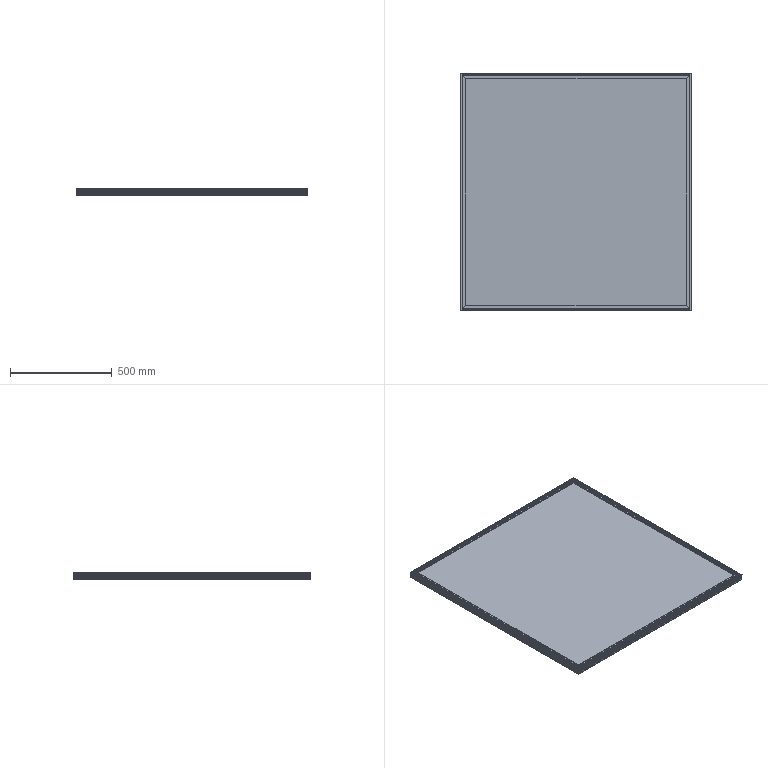Part | 5 solids | 272 faces | box 1140 x 1170 x 30 mm | volume 21812223 mm3 | plane 222 | cylinder 50 | commonest cylinder face diameters 0.4 x26 2 x16 1 x8